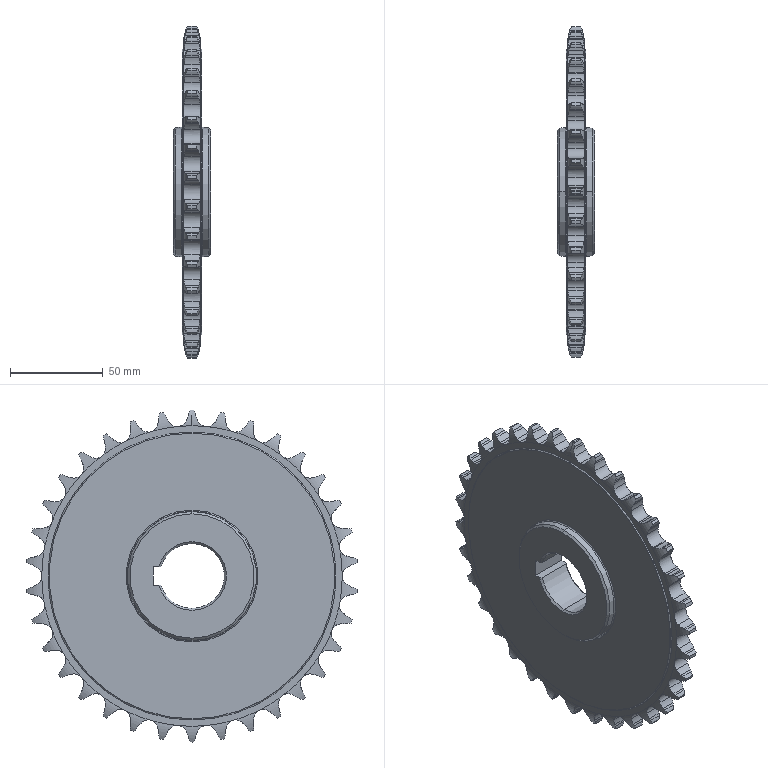Part | SolidWorks | features Cut 2, Revolution 2, Chamfer 1, CirPattern 1, Fillet 1, MirrorPattern 1 | 1 solid | 399 faces | box 20 x 178.394 x 179 mm | volume 238483 mm3 | cylinder 230 | torus 78 | plane 77 | cone 14 | commonest cylinder face diameters 14.533 x72 26.567 x72 10.311 x44 179 x35 154 x4 35 x3